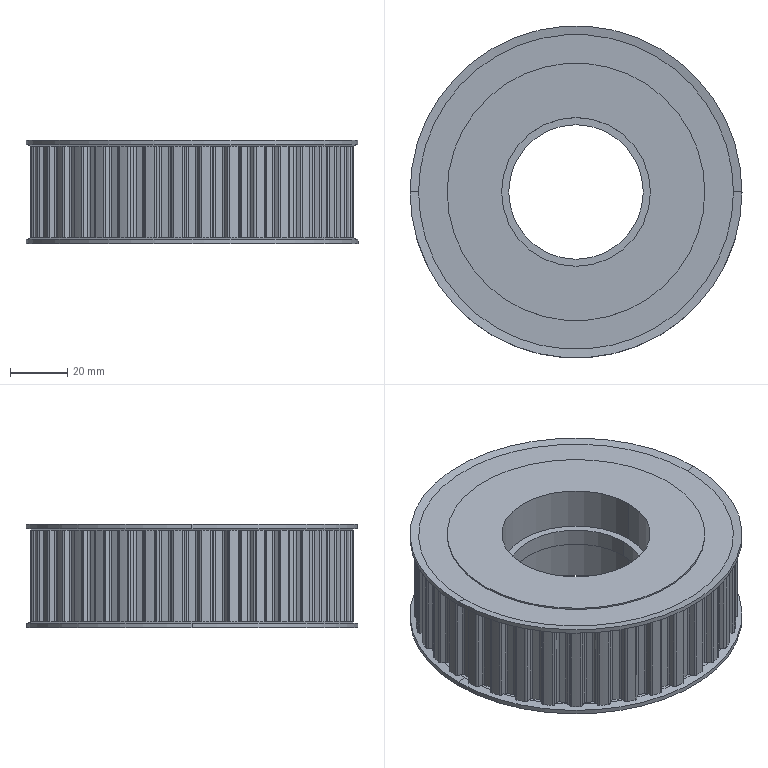Part | SolidWorks | features BaseBody 3 | 3 solids | 350 faces | box 116 x 116 x 36 mm | volume 270437 mm3 | cylinder 224 | plane 118 | cone 8 | commonest cylinder face diameters 1.6 x170 112.75 x36 90 x8 52 x4 116 x4 47 x2